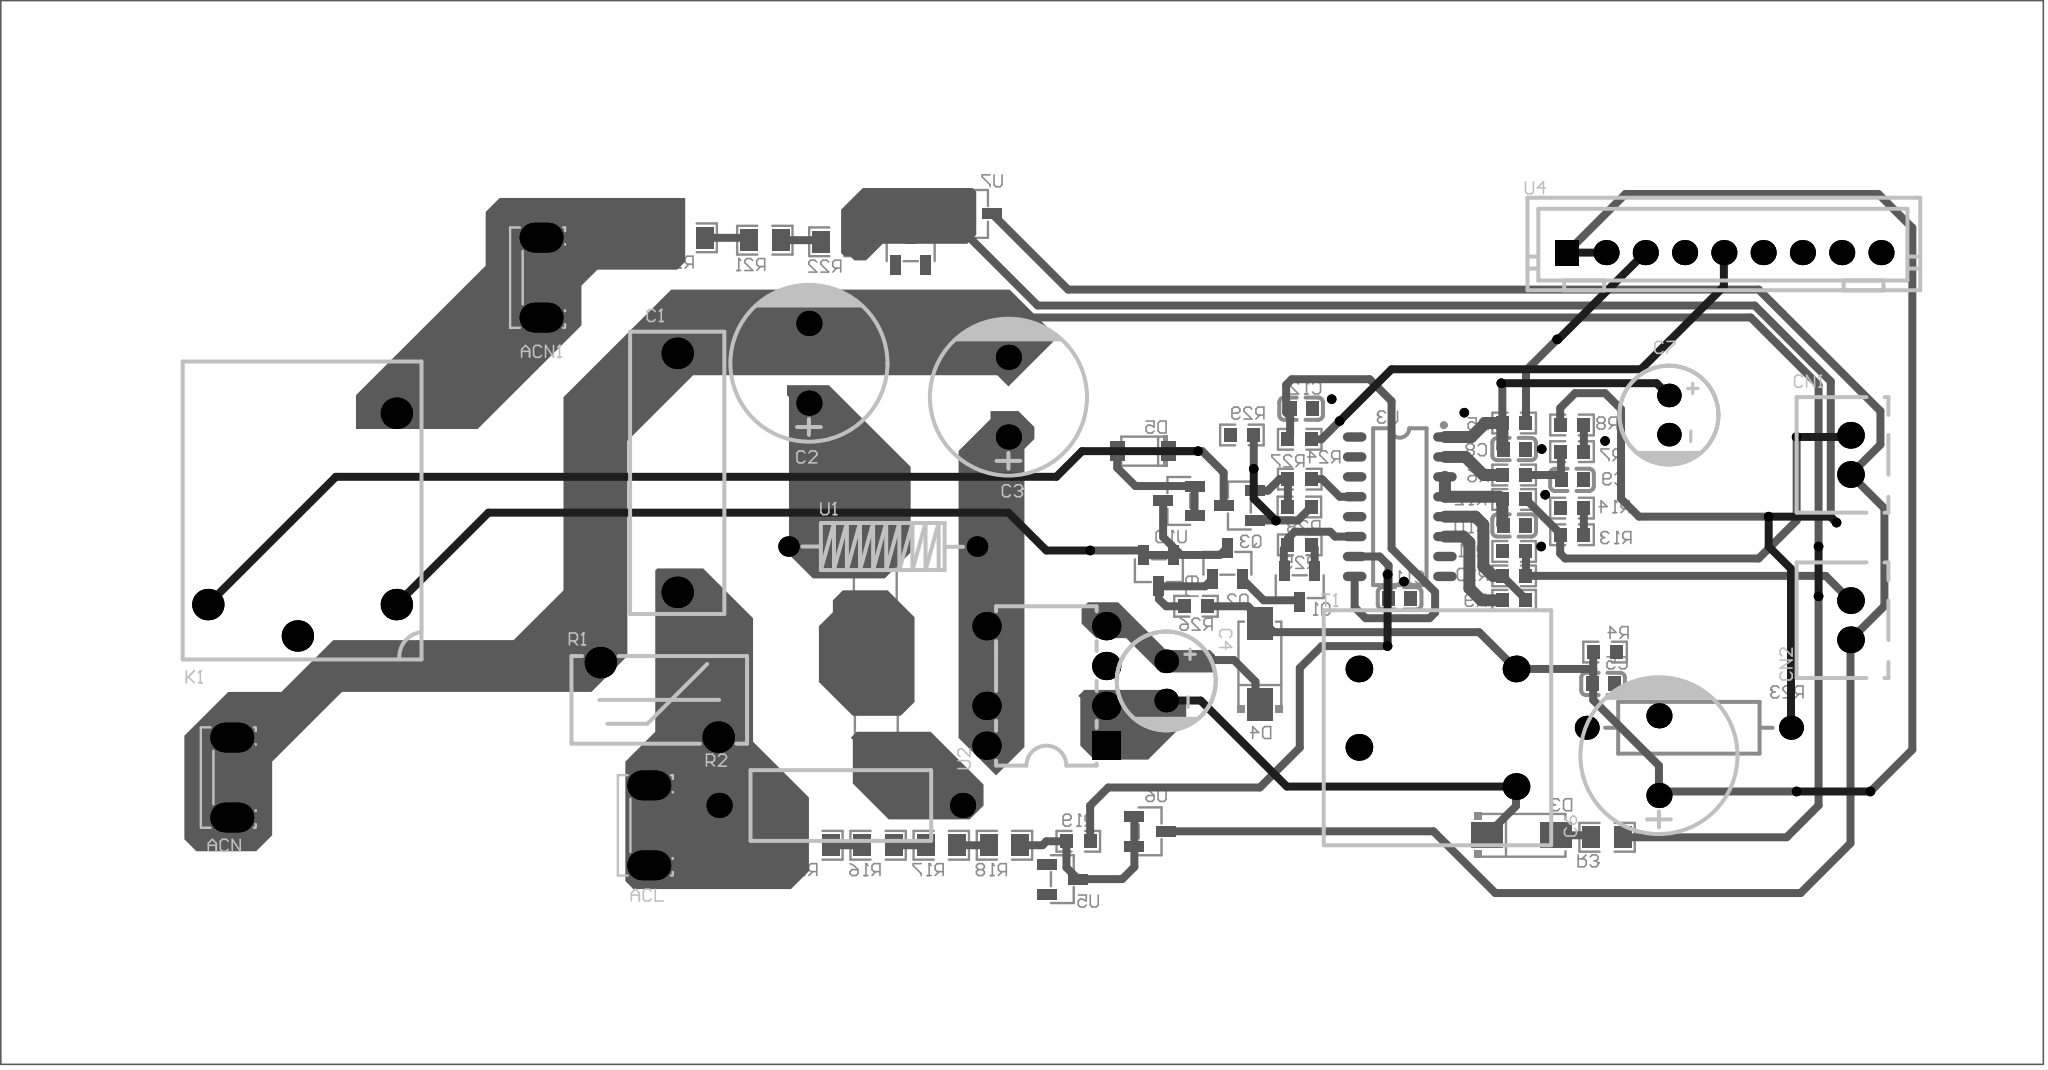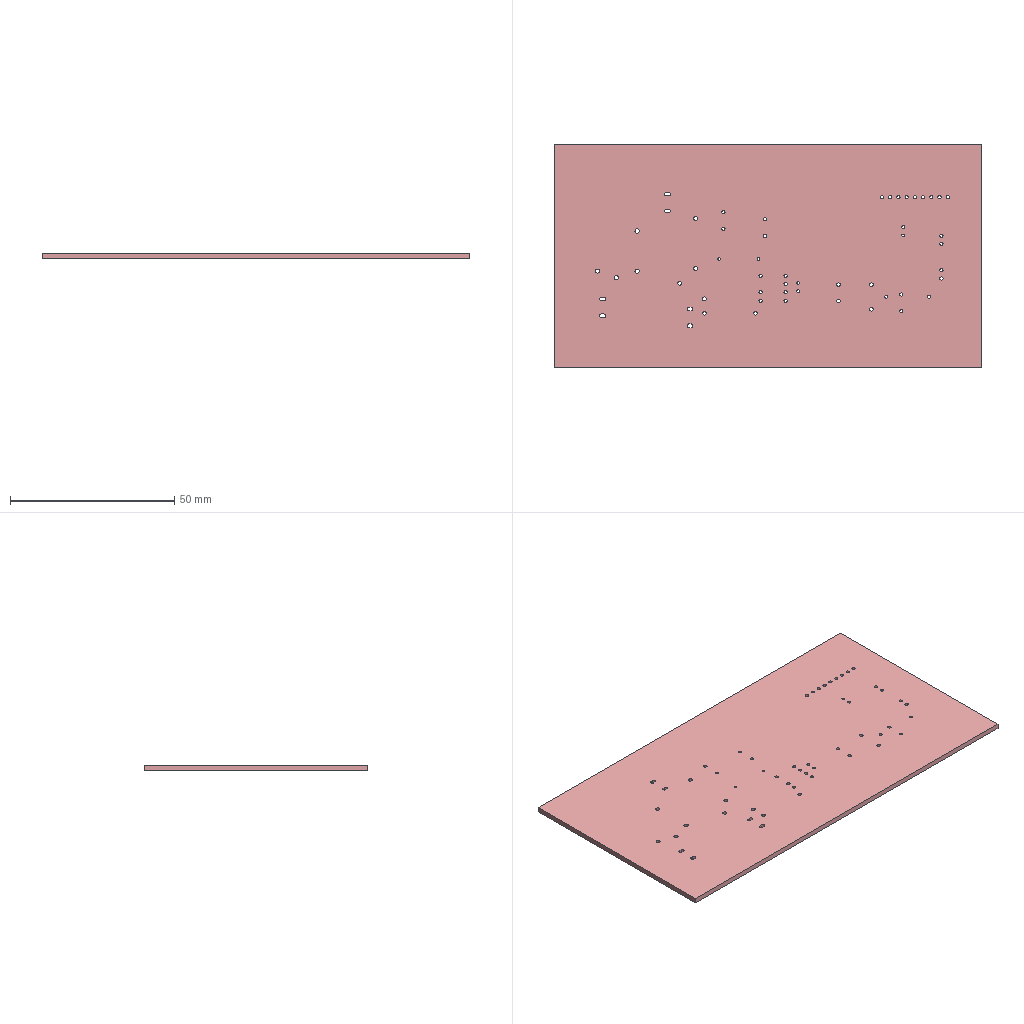Circuit board layout | Altium Designer | box 130 x 67.8 x 1.6 mm
Layer stack:
# Altium Designer layer stack of  (unit mm; dielectric type: 0 none, 1 core, 2 prepreg, 3 surface material)
index,name,kind,layer,copper_thickness_mm,dielectric_type,dielectric_thickness_mm,dielectric_material,dielectric_constant
0,Top Paste Mask Layer,other,,,,,,
1,Top Silkscreen Layer,other,,,,,,
2,Top Solder Mask Layer,dielectric,,,3,0.01,,3.3
3,Top Layer,copper,Top Layer,0.035,,,,
4,Dielectric1,dielectric,,,3,1.51,FR4,4.5
5,Bottom Layer,copper,Bottom Layer,0.035,,,,
6,Bottom Solder Mask Layer,dielectric,,,3,0.01,,3.3
7,Bottom Silkscreen Layer,other,,,,,,
8,Bottom Paste Mask Layer,other,,,,,,
# drill layer pairs: low layer,high layer
drill_pair,Top Layer,Bottom Layer
Part placement:
Designator,Comment,Layer,Footprint,Center-X(mm),Center-Y(mm),Rotation
ACL,T250036-3B80,TopLayer,CONN-TH_XFCN-T250036-3B80,111.125,85.09,90
ACN,T250036-3B80,TopLayer,CONN-TH_XFCN-T250036-3B80,84.582,88.138,90
ACN1,T250036-3B80,TopLayer,CONN-TH_XFCN-T250036-3B80,104.267,120.015,90
C1,100nF,TopLayer,CAP-TH_L18.0-W6.0-P15.00-D1.2,112.903,107.569,270
C2,4.7uF,TopLayer,CAP-TH_BD10.0-P5.00-D1.0-FD,121.285,114.554,90
C3,4.7uF,TopLayer,CAP-TH_BD10.0-P5.00-D1.0-FD,133.985,112.395,90
C4,4.7uF,TopLayer,CAP-TH_BD6.3-P2.50-D0.5-FD,144.028,94.299,270
C5,100nF,BottomLayer,C0603,171.831,94.107,180
C6,470uF,TopLayer,CAP-TH_BD10.0-P5.00-D1.0-FD,175.387,89.535,90
C7,100uF,TopLayer,CAP-TH_BD6.3-P2.50-D0.5-FD,176.022,111.252,270
C8,1uF,BottomLayer,C0603,166.172,109.086,0
C9,1uF,BottomLayer,C0603,169.855,107.12,0
C10,100nF,BottomLayer,C0603,166.172,104.213,180
C11,100nF,BottomLayer,C0603,158.881,99.566,180
C12,100nF,BottomLayer,C0603,152.612,111.659,0
CN1,B2B-XH-A(LF)(SN),TopLayer,CONN-TH_B2B-XH-A-LF-SN,187.579,108.712,90
CN2,B2B-XH-A(LF)(SN),TopLayer,CONN-TH_B2B-XH-A-LF-SN,187.579,98.171,90
D1,US1M,BottomLayer,SMA_L4.4-W2.8-LS5.4-RD,125.575,92.296,270
D2,US1M,BottomLayer,SMA_L4.4-W2.8-LS5.4-RD,125.509,101.064,270
D3,BYV26C,BottomLayer,SMA_L4.4-W2.6-LS5.1-FD,166.624,84.455,180
D4,US1M,BottomLayer,SMA_L4.4-W2.8-LS5.4-RD,149.987,95.377,90
D5,MMSZ5242B,BottomLayer,SOD-123_L2.7-W1.6-LS3.7-RD,142.543,108.951,180
K1,HF3FF-012-1HST,TopLayer,RELAY-TH_HF3FF-012-1HST,89.027,104.267,90
Q1,SS8050,BottomLayer,SOT-23-3_L2.9-W1.3-P1.90-LS2.4-BR,152.524,100.309,90
Q2,SS8050,BottomLayer,SOT-23-3_L2.9-W1.3-P1.90-LS2.4-BR,147.921,101.799,270
Q3,SS8050,BottomLayer,SOT-23-3_L2.9-W1.3-P1.90-LS2.4-BR,148.683,105.482,0
R1,180pF,TopLayer,RES-TH_L11.0-W5.5-P7.50-D0.8-S4.70,111.76,93.091,0
R2,2.2kΩ,TopLayer,RES-TH_BD4.5-L11.5-P15.50-D0.8,123.317,86.36,0
R3,0Ω,BottomLayer,R0805,172.085,84.328,0
R4,10kΩ,BottomLayer,R0603,171.958,96.139,180
R5,1kΩ,BottomLayer,R0603,166.172,110.744,0
R6,1kΩ,BottomLayer,R0603,166.172,107.429,0
R7,1kΩ,BottomLayer,R0603,169.855,108.92,0
R8,10kΩ,BottomLayer,R0603,169.855,110.62,180
R9,1kΩ,BottomLayer,R0603,166.172,99.441,0
R10,10kΩ,BottomLayer,R0603,166.172,100.998,180
R11,5.1kΩ,BottomLayer,R0603,166.172,102.556,180
R12,10kΩ,BottomLayer,R0603,166.172,105.871,180
R13,5.1kΩ,BottomLayer,R0603,169.855,103.62,0
R14,1kΩ,BottomLayer,R0603,169.855,105.32,0
R15,240kΩ,BottomLayer,R0805,121.666,83.82,0
R16,240kΩ,BottomLayer,R0805,125.688,83.82,0
R17,240kΩ,BottomLayer,R0805,129.709,83.82,0
R18,240kΩ,BottomLayer,R0805,133.731,83.82,0
R19,10kΩ,BottomLayer,R0603,138.43,84.074,0
R20,150kΩ,BottomLayer,R0805,113.665,122.555,0
R21,150kΩ,BottomLayer,R0805,118.479,122.403,0
R22,180kΩ,BottomLayer,R0805,123.063,122.301,0
R23,4.7kΩ,BottomLayer,RES-TH_BD3.3-L9.0-P13.00-D0.6,177.292,91.313,180
R24,100Ω,BottomLayer,R0603,152.524,109.707,180
R25,4.7K,BottomLayer,R0603,152.524,102.976,0
R26,4.7K,BottomLayer,R0603,145.923,99.06,0
R27,4.7kΩ,BottomLayer,R0603,152.524,107.167,0
R28,4.7kΩ,BottomLayer,R0603,152.503,105.391,180
R29,10kΩ,BottomLayer,R0603,148.844,109.982,0
T1,XREE14-250408,TopLayer,XFMR-TH_XREE14-250408,161.29,91.313,0
U1,1mH,TopLayer,IND-TH_BD3.0-L8.0-P12.00-D0.6,125.984,102.87,0
U2,PN8034NSC-T1,TopLayer,DIP-8_7P-L9.3-W6.4-P2.54-LS7.6-BL-PE6,136.398,93.98,90
U3,CMS79F123,BottomLayer,SOPN-16_L9.9-W3.9-P1.27-LS6.0-BL,158.893,105.408,270
U4,ZX-XH2.54-9PZZ,TopLayer,CONN-TH_9P-P2.50_ZX-XH2.54-9PZZ,179.519,121.612,0
U5,MMBD4148,BottomLayer,SOT-23-3_L2.9-W1.3-P1.90-LS2.4-BR,137.414,81.661,180
U6,MMBD4148,BottomLayer,SOT-23-3_L2.9-W1.3-P1.90-LS2.4-BR,143.002,84.709,180
U7,MMBD4148,BottomLayer,SOT-23-3_L2.9-W1.3-P1.90-LS2.4-BR,131.953,124.079,180
U8,MMBD4148,BottomLayer,SOT-23-3_L2.9-W1.3-P1.90-LS2.4-BR,127.762,121.793,270
U9,MMBD4148,BottomLayer,SOT-23-3_L2.9-W1.3-P1.90-LS2.4-BR,143.559,101.331,90
U10,MMBD4148,BottomLayer,SOT-23-3_L2.9-W1.3-P1.90-LS2.4-BR,144.829,105.776,0
Pad and via stacks:
# Altium Designer via and pad stacks of  (unit mm). Each distinct definition once, with the count of objects using it.
# via: kind,start_layer,end_layer,hole_mm,diameter_mm,mode(0 simple;1 top-mid-bottom;2 full stack),diameter_per_layer,count,example_net
# pad: kind,layer,hole_mm,hole_type(0 round;1 square;2 slot),plating,top_size,top_shape(1 round;2 rect;3 octagon;9 rounded rect),mid_size,bottom_size,mode,footprint,size_per_layer,count,example
pad,Multi-Layer,1.1,2,plated,2.8x1.9,1,2.8x1.9,2.8x1.9,0,CONN-TH_XFCN-T250036-3B80,,6,ACL.1
pad,Multi-Layer,1.2,0,plated,2x2,1,2x2,2x2,0,CAP-TH_L18.0-W6.0-P15.00-D1.2,,2,C1.1
pad,Multi-Layer,1,0,plated,1.6x1.6,1,1.6x1.6,1.6x1.6,0,CAP-TH_BD10.0-P5.00-D1.0-FD,,6,C2.1
pad,Multi-Layer,0.9,0,plated,1.5x1.5,1,1.5x1.5,1.5x1.5,0,CAP-TH_BD6.3-P2.50-D0.5-FD,,4,C4.2
pad,Multi-Layer,1,0,plated,1.7x1.7,1,1.7x1.7,1.7x1.7,0,CONN-TH_B2B-XH-A-LF-SN,,4,CN1.1
pad,Multi-Layer,1.3,0,plated,2x2,1,2x2,2x2,0,RELAY-TH_HF3FF-012-1HST,,4,K1.4
pad,Multi-Layer,1.2,0,plated,2x2,1,2x2,2x2,0,RES-TH_L11.0-W5.5-P7.50-D0.8-S4.70,,2,R1.1
pad,Multi-Layer,1.1,0,plated,1.6x1.6,1,1.6x1.6,1.6x1.6,0,RES-TH_BD4.5-L11.5-P15.50-D0.8,,2,R2.1
pad,Multi-Layer,0.9144,0,plated,1.524x1.524,1,1.524x1.524,1.524x1.524,0,RES-TH_BD3.3-L9.0-P13.00-D0.6,,2,R23.2
pad,Multi-Layer,1.1,0,plated,1.7x1.7,1,1.7x1.7,1.7x1.7,0,XFMR-TH_XREE14-250408,,4,T1.1
pad,Multi-Layer,0.8,0,plated,1.3x1.3,1,1.3x1.3,1.3x1.3,0,IND-TH_BD3.0-L8.0-P12.00-D0.6,,2,U1.1
pad,Multi-Layer,1,0,plated,1.8x1.8,1,1.8x1.8,1.8x1.8,0,DIP-8_7P-L9.3-W6.4-P2.54-LS7.6-BL-PE6,,6,U2.7
pad,Multi-Layer,1,0,plated,1.8x1.8,2,1.8x1.8,1.8x1.8,0,DIP-8_7P-L9.3-W6.4-P2.54-LS7.6-BL-PE6,,1,U2.1
pad,Multi-Layer,1,0,plated,1.524x1.6,2,1.524x1.6,1.524x1.6,0,CONN-TH_9P-P2.50_ZX-XH2.54-9PZZ,,1,U4.1
pad,Multi-Layer,1,0,plated,1.6x1.6,1,1.6x1.6,1.6x1.6,0,CONN-TH_9P-P2.50_ZX-XH2.54-9PZZ,,8,U4.2
pad,Bottom Layer,0,0,plated,0.8x0.9,2,0.8x0.9,0.8x0.9,0,C0603,,12,C5.2
pad,Bottom Layer,0,0,plated,2.046x1.62,2,2.046x1.62,2.046x1.62,0,SMA_L4.4-W2.8-LS5.4-RD,,6,D1.2
pad,Bottom Layer,0,0,plated,2x1.62,2,2x1.62,2x1.62,0,SMA_L4.4-W2.6-LS5.1-FD,,2,D3.2
pad,Bottom Layer,0,0,plated,0.91x1.22,2,0.91x1.22,0.91x1.22,0,SOD-123_L2.7-W1.6-LS3.7-RD,,2,D5.2
pad,Bottom Layer,0,0,plated,1.25x0.7,2,1.25x0.7,1.25x0.7,0,SOT-23-3_L2.9-W1.3-P1.90-LS2.4-BR,,27,Q1.1
pad,Bottom Layer,0,0,plated,1.133x1.377,2,1.133x1.377,1.133x1.377,0,R0805,,16,R3.2
pad,Bottom Layer,0,0,plated,0.8065x0.864,2,0.8065x0.864,0.8065x0.864,0,R0603,,36,R4.2
pad,Bottom Layer,0,0,plated,1.508x0.6,1,1.508x0.6,1.508x0.6,0,SOPN-16_L9.9-W3.9-P1.27-LS6.0-BL,,16,U3.1
via,Top Layer,Bottom Layer,0.3048,0.61,0,,23,$1N73